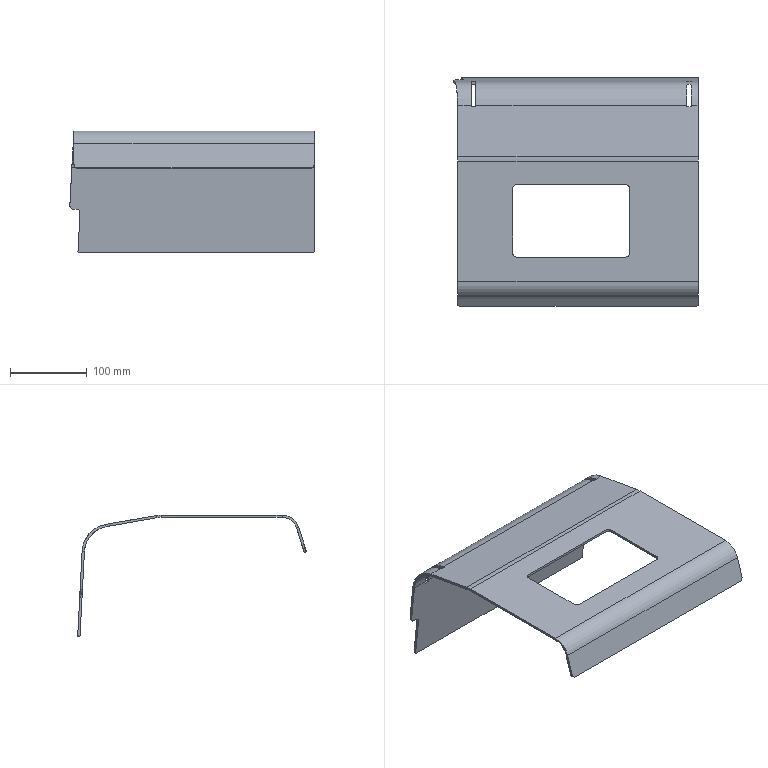Part | SolidWorks | features Fillet 2, ICE 2, FlatPattern 1, Fold 1, SMBaseFlange 1, SheetMetal 1, UnFold 1 | 1 solid | 68 faces | box 317.63 x 297.4 x 158.457 mm | volume 376681 mm3 | plane 46 | cylinder 21 | spline 1 | commonest cylinder face diameters 10 x9 68 x4 74 x4 4 x2 40 x1 46 x1